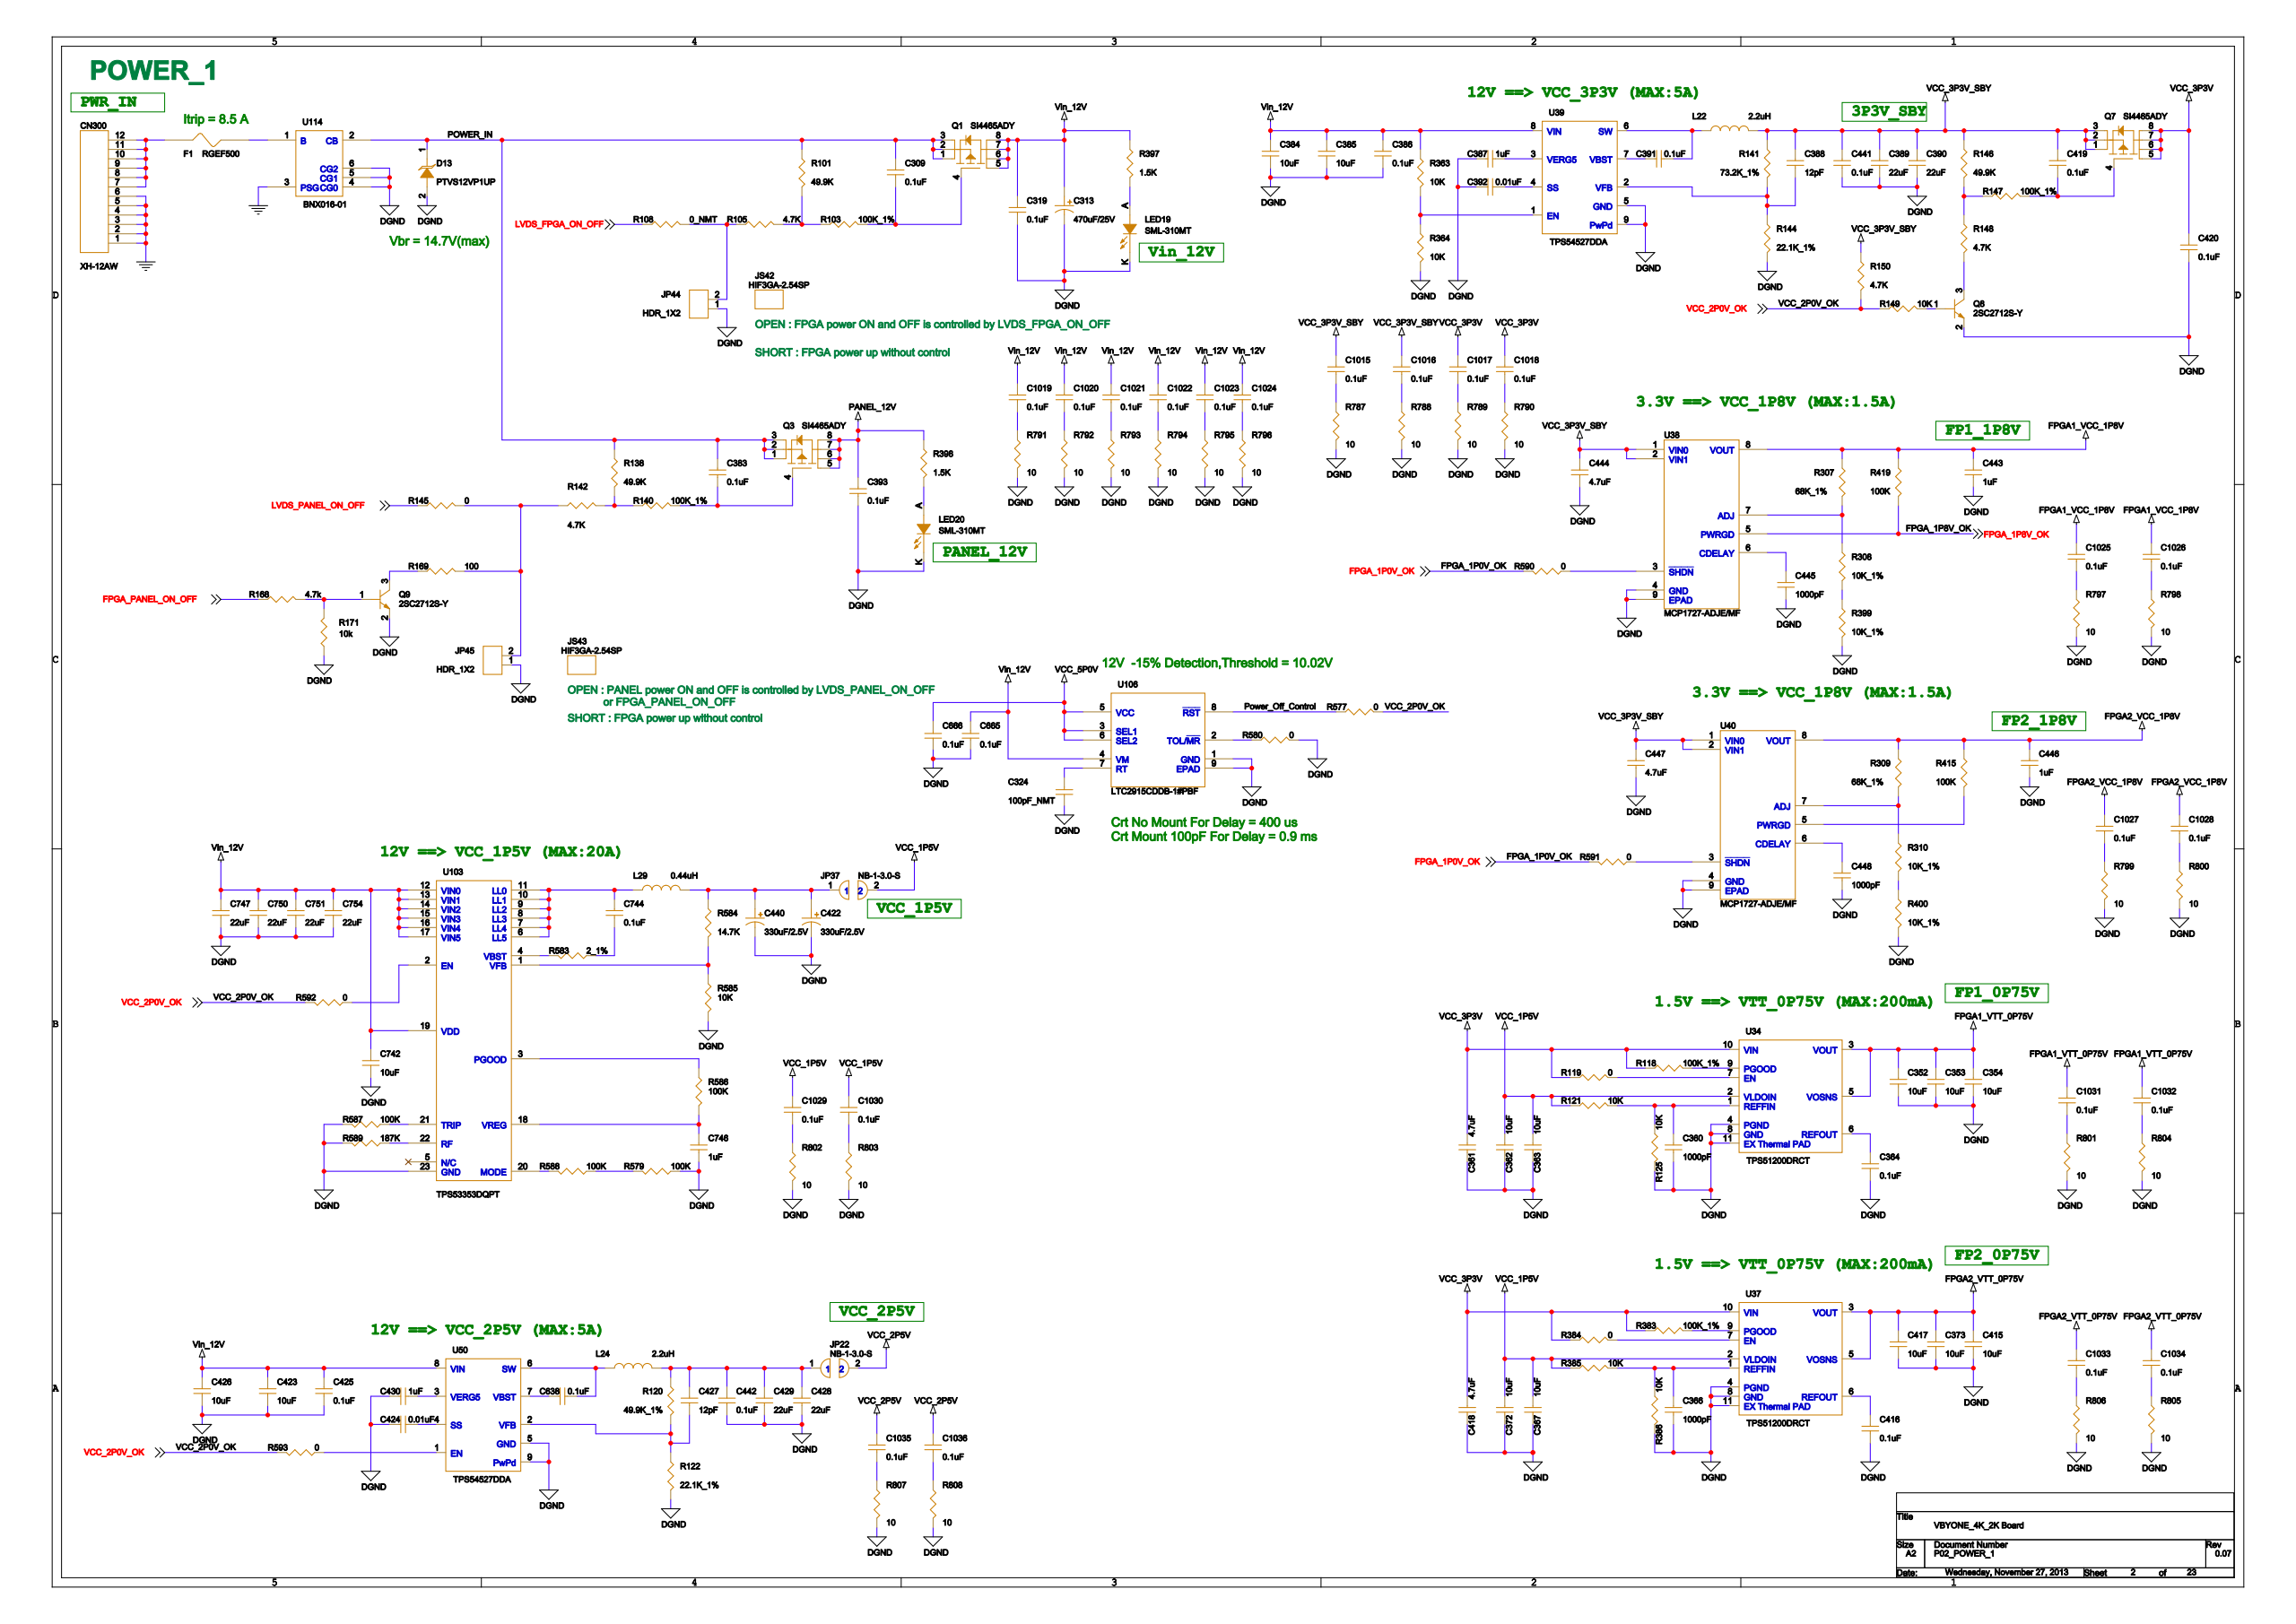Circuit board | Cadence Allegro | 1712 parts | 1495 nets | one sheet of the schematic
Parts on this sheet (reference | value | footprint):
C309 | 0.1uF | CRC1005RZAS
C313 | 470uF/25V | CEC100RZAS
C319 | 0.1uF | CRC1005RZAS
C324 | 100pF_NMT | CRC1608RZAS
C352 | 10uF | CRC2012RZAS
C353 | 10uF | CRC2012RZAS
C354 | 10uF | CRC2012RZAS
C360 | 1000pF | CRC1608RZAS
C361 | 4.7uF | CRC1608RZAS
C362 | 10uF | CRC2012RZAS
C363 | 10uF | CRC2012RZAS
C364 | 0.1uF | CRC1005RZAS
C366 | 1000pF | CRC1608RZAS
C367 | 10uF | CRC2012RZAS
C372 | 10uF | CRC2012RZAS
C373 | 10uF | CRC2012RZAS
C383 | 0.1uF | CRC1005RZAS
C384 | 10uF | CRC2012RZAS
C385 | 10uF | CRC2012RZAS
C386 | 0.1uF | CRC1005RZAS
C387 | 1uF | CRC1608RZAS
C388 | 12pF | CRC1608RZAS
C389 | 22uF | CRC3225RZAS
C390 | 22uF | CRC3225RZAS
C391 | 0.1uF | CRC1005RZAS
C392 | 0.01uF | CRC1005RZAS
C393 | 0.1uF | CRC1005RZAS
C415 | 10uF | CRC2012RZAS
C416 | 0.1uF | CRC1005RZAS
C417 | 10uF | CRC2012RZAS
C418 | 4.7uF | CRC1608RZAS
C419 | 0.1uF | CRC1005RZAS
C420 | 0.1uF | CRC1005RZAS
C422 | 330uF/2.5V | CEC3528RZAS
C423 | 10uF | CRC2012RZAS
C424 | 0.01uF | CRC1005RZAS
C425 | 0.1uF | CRC1005RZAS
C426 | 10uF | CRC2012RZAS
C427 | 12pF | CRC1608RZAS
C428 | 22uF | CRC3225RZAS
C429 | 22uF | CRC3225RZAS
C430 | 1uF | CRC1608RZAS
C440 | 330uF/2.5V | CEC3528RZAS
C441 | 0.1uF | CRC1005RZAS
C442 | 0.1uF | CRC1005RZAS
C443 | 1uF | CRC1608RZAS
C444 | 4.7uF | CRC1608RZAS
C445 | 1000pF | CRC1608RZAS
C446 | 1uF | CRC1608RZAS
C447 | 4.7uF | CRC1608RZAS
C448 | 1000pF | CRC1608RZAS
C638 | 0.1uF | CRC1005RZAS
C665 | 0.1uF | CRC1005RZAS
C666 | 0.1uF | CRC1005RZAS
C742 | 10uF | CRC2012RZAS
C744 | 0.1uF | CRC1005RZAS
C746 | 1uF | CRC1608RZAS
C747 | 22uF | CRC3225RZAS
C750 | 22uF | CRC3225RZAS
C751 | 22uF | CRC3225RZAS
C754 | 22uF | CRC3225RZAS
C1015 | 0.1uF | CRC1005RZAS
C1016 | 0.1uF | CRC1005RZAS
C1017 | 0.1uF | CRC1005RZAS
C1018 | 0.1uF | CRC1005RZAS
C1019 | 0.1uF | CRC1005RZAS
C1020 | 0.1uF | CRC1005RZAS
C1021 | 0.1uF | CRC1005RZAS
C1022 | 0.1uF | CRC1005RZAS
C1023 | 0.1uF | CRC1005RZAS
C1024 | 0.1uF | CRC1005RZAS
C1025 | 0.1uF | CRC1005RZAS
C1026 | 0.1uF | CRC1005RZAS
C1027 | 0.1uF | CRC1005RZAS
C1028 | 0.1uF | CRC1005RZAS
C1029 | 0.1uF | CRC1005RZAS
C1030 | 0.1uF | CRC1005RZAS
C1031 | 0.1uF | CRC1005RZAS
C1032 | 0.1uF | CRC1005RZAS
C1033 | 0.1uF | CRC1005RZAS
C1034 | 0.1uF | CRC1005RZAS
C1035 | 0.1uF | CRC1005RZAS
C1036 | 0.1uF | CRC1005RZAS
CN300 | XH-12AW | CAD012LKAS
D13 | PTVS12VP1UP | DIC002RZIS-2
F1 | RGEF500 | FLD002RZBS
JP22 | NB-1-3.0-S | CUTLAND35
JP37 | NB-1-3.0-S | CUTLAND35
JP44 | HDR_1X2 | CND002LLBS
JP45 | HDR_1X2 | CND002LLBS
L22 | 2.2uH | LSC5247RZAS
L24 | 2.2uH | LSC5247RZAS
L29 | 0.44uH | LSC002RZOS
LED19 | SML-310MT | LEC1608RZAS
LED20 | SML-310MT | LEC1608RZAS
Q1 | SI4465ADY | SOC008RHAS
Q3 | SI4465ADY | SOC008RHAS
Q7 | SI4465ADY | SOC008RHAS
Q8 | 2SC2712S-Y | TRC003RZCS
Q9 | 2SC2712S-Y | TRC003RZCS
R101 | 49.9K | CRC1608RZAS
R103 | 100K_1% | CRC1608RZAS
R105 | 4.7K | CRC1005RZAS
R108 | 0_NMT | CRC1608RZAS
R118 | 100K_1% | CRC1608RZAS
R119 | 0 | CRC1608RZAS
R120 | 49.9K_1% | CRC1608RZAS
R121 | 10K | CRC1005RZAS
R122 | 22.1K_1% | CRC1608RZAS
R125 | 10K | CRC1005RZAS
R138 | 49.9K | CRC1608RZAS
R140 | 100K_1% | CRC1608RZAS
R141 | 73.2K_1% | CRC1608RZAS
R142 | 4.7K | CRC1005RZAS
R144 | 22.1K_1% | CRC1608RZAS
R145 | 0 | CRC1608RZAS
R146 | 49.9K | CRC1608RZAS
R147 | 100K_1% | CRC1608RZAS
R148 | 4.7K | CRC1005RZAS
R149 | 10K | CRC1005RZAS
R150 | 4.7K | CRC1005RZAS
R168 | 4.7K | CRC1005RZAS
R169 | 100 | CRC1005RZAS
R171 | 10K | CRC1005RZAS
R307 | 68K_1% | CRC1608RZAS
R308 | 10K_1% | CRC1005RZAS
R309 | 68K_1% | CRC1608RZAS
R310 | 10K_1% | CRC1005RZAS
R363 | 10K | CRC1005RZAS
R364 | 10K | CRC1005RZAS
R383 | 100K_1% | CRC1608RZAS
R384 | 0 | CRC1608RZAS
R385 | 10K | CRC1005RZAS
R386 | 10K | CRC1005RZAS
R397 | 1.5K | CRC1608RZAS
R398 | 1.5K | CRC1608RZAS
R399 | 10K_1% | CRC1005RZAS
R400 | 10K_1% | CRC1005RZAS
R415 | 100K | CRC1608RZAS
R419 | 100K | CRC1608RZAS
R577 | 0 | CRC1608RZAS
R579 | 100K | CRC1608RZAS
R580 | 0 | CRC1608RZAS
R583 | 2_1% | CRC1608RZAS
R584 | 14.7K | CRC1608RZAS
R585 | 10K | CRC1005RZAS
R586 | 100K | CRC1608RZAS
R587 | 100K | CRC1608RZAS
R588 | 100K | CRC1608RZAS
R589 | 187K | CRC1608RZAS
R590 | 0 | CRC1608RZAS
R591 | 0 | CRC1608RZAS
R592 | 0 | CRC1608RZAS
R593 | 0 | CRC1608RZAS
R787 | 10 | CRC1005RZAS
R788 | 10 | CRC1005RZAS
R789 | 10 | CRC1005RZAS
R790 | 10 | CRC1005RZAS
R791 | 10 | CRC1005RZAS
R792 | 10 | CRC1005RZAS
R793 | 10 | CRC1005RZAS
R794 | 10 | CRC1005RZAS
R795 | 10 | CRC1005RZAS
R796 | 10 | CRC1005RZAS
R797 | 10 | CRC1005RZAS
R798 | 10 | CRC1005RZAS
R799 | 10 | CRC1005RZAS
R800 | 10 | CRC1005RZAS
R801 | 10 | CRC1005RZAS
R802 | 10 | CRC1005RZAS
R803 | 10 | CRC1005RZAS
R804 | 10 | CRC1005RZAS
R805 | 10 | CRC1005RZAS
R806 | 10 | CRC1005RZAS
R807 | 10 | CRC1005RZAS
R808 | 10 | CRC1005RZAS
U34 | TPS51200DRCT | QFN010RCAS
U37 | TPS51200DRCT | QFN010RCAS
U38 | MCP1727-ADJE/MF | SOC008REDS
U39 | TPS54527DDA | SOC008RHBS
U40 | MCP1727-ADJE/MF | SOC008REDS
U50 | TPS54527DDA | SOC008RHBS
U103 | TPS53353DQPT | SOC022RCAS
U106 | LTC2915CDDB-1#PBF | SOC008RCDS
U114 | BNX016-01 | FLD006LKAS
Nets of these parts (net: part-pin ...):
VCC_3P3V: C361-1 C418-1 C420-1 C1017-1 C1018-1 Q7-5 Q7-6 Q7-7 Q7-8 R118-1 R119-1 R383-1 R384-1 U34-10 U37-10
DGND: C313-2 C319-2 C324-1 C352-2 C353-2 C354-2 C360-2 C361-2 C362-2 C363-2 C364-2 C366-2 C367-2 C372-2 C373-2 C384-2 C385-2 C386-2 C387-1 C389-2 C390-2 C392-1 C393-2 C415-2 C416-2 C417-2 C418-2 C420-2 C422-2 C423-2 C424-1 C425-2 C426-2 C428-2 C429-2 C430-1 C440-2 C441-2 C442-2 C443-2 C444-2 C445-2 C446-2 C447-2 C448-2 C665-1 C666-1 C742-2 C746-2 C747-2 C750-2 C751-2 C754-2 D13-2 JP44-1 JP45-1 LED19-K LED20-K Q8-2 Q9-2 R122-2 R125-2 R144-2 R171-1 R364-2 R386-2 R399-2 R400-2 R579-1 R580-2 R585-2 R587-2 R589-2 R787-2 R788-2 R789-2 R790-2 R791-2 R792-2 R793-2 R794-2 R795-2 R796-2 R797-2 R798-2 R799-2 R800-2 R801-2 R802-2 R803-2 R804-2 R805-2 R806-2 R807-2 R808-2 U34-4 U34-8 U34-11 U37-4 U37-8 U37-11 U38-4 U38-9 U39-5 U39-9 U40-4 U40-9 U50-5 U50-9 U106-1 U106-9 U114-4 U114-5 U114-6 U103-23
VCC_1P5V: C362-1 C363-1 C367-1 C372-1 C1029-1 C1030-1 JP37-2 R121-1 R385-1 U34-2 U37-2
VCC_3P3V_SBY: C388-1 C389-1 C390-1 C419-1 C441-1 C444-1 C447-1 C1015-1 C1016-1 L22-2 Q7-1 Q7-2 Q7-3 R141-1 R146-1 R150-1 U38-1 U38-2 U40-1 U40-2
N19944978: C1015-2 R787-1
N19945009: C1016-2 R788-1
N19945053: C1017-2 R789-1
N19945065: C1018-2 R790-1
VIN_12V: C313-1 C319-1 C384-1 C385-1 C386-1 C423-1 C425-1 C426-1 C665-2 C742-1 C747-1 C750-1 C751-1 C754-1 C1019-1 C1020-1 C1021-1 C1022-1 C1023-1 C1024-1 Q1-5 Q1-6 Q1-7 Q1-8 R363-1 R397-1 U39-8 U50-8 U106-4 U103-12 U103-13 U103-14 U103-15 U103-16 U103-17 U103-19
N19940256: C1019-2 R791-1
N19941245: C1020-2 R792-1
N19941511: C1021-2 R793-1
N19941779: C1022-2 R794-1
N19941808: C1023-2 R795-1
N19941837: C1024-2 R796-1
FPGA1_VCC_1P8V: C443-1 C1025-1 C1026-1 R307-1 R419-1 U38-8
N19947558: C1025-2 R797-1
N19947572: C1026-2 R798-1
FPGA2_VCC_1P8V: C446-1 C1027-1 C1028-1 R309-1 R415-1 U40-8
N19948575: C1027-2 R799-1
N19948579: C1028-2 R800-1
N19951656: C1029-2 R802-1
N19951688: C1030-2 R803-1
FPGA1_VTT_0P75V: C352-1 C353-1 C354-1 C1031-1 C1032-1 U34-3 U34-5
N19948889: C1031-2 R801-1
N19948895: C1032-2 R804-1
FPGA2_VTT_0P75V: C373-1 C415-1 C417-1 C1033-1 C1034-1 U37-3 U37-5
N19949219: C1033-2 R806-1
N19949213: C1034-2 R805-1
VCC_2P5V: C1035-1 C1036-1 JP22-2
N19951132: C1035-2 R807-1
N19951164: C1036-2 R808-1
POWER_IN: C309-1 C383-1 D13-1 Q1-1 Q1-2 Q1-3 Q3-1 Q3-2 Q3-3 R101-1 R138-1 U114-2
N15783925: C309-2 Q1-4 R103-2
N16970548: C364-1 U34-6
N17163997: C383-2 Q3-4 R140-2
N17322746: C391-1 U39-7
N17322740: C391-2 L22-1 U39-6
PANEL_12V: C393-1 Q3-5 Q3-6 Q3-7 Q3-8 R398-1
N18162801: C416-1 U37-6
N17546760: C419-2 Q7-4 R147-2
N18317834: C427-1 C428-1 C429-1 C442-1 JP22-1 L24-2 R120-1
N18317826: C638-1 U50-7
N18317824: C638-2 L24-1 U50-6
VCC_5P0V: C666-2 U106-3 U106-5 U106-6
N17322991: C387-2 U39-3
N18317806: C430-2 U50-3
N16970580: C360-1 R121-2 R125-1 U34-1
N18162813: C366-1 R385-2 R386-1 U37-1
N18318720: C445-1 U38-6
N18320450: C448-1 U40-6
N18312599: C744-1 L29-1 U103-6 U103-7 U103-8 U103-9 U103-10 U103-11
N18312643: C744-2 R583-1
N18161409: C324-2 U106-7
N18312681: C746-1 R586-2 U103-18
N17322734: C388-2 R141-2 R144-1 U39-2
N18317842: C427-2 R120-2 R122-1 U50-2
N17322989: C392-2 U39-4
N18317822: C424-2 U50-4
N18312559: C422-1 C440-1 JP37-1 L29-2 R584-1
LVDS_PANEL_ON_OFF: R145-1
LVDS_FPGA_ON_OFF: R108-1
GND: CN300-1 CN300-2 CN300-3 CN300-4 CN300-5 CN300-6 U114-3
N15783757: CN300-7 CN300-8 CN300-9 CN300-10 CN300-11 CN300-12 F1-1
N18434432: F1-2 U114-1
N18311244: JP44-2 R105-1 R108-2
N18311238: JP45-2 R142-1 R145-2 R169-2
N18306479: LED19-A R397-2
N18307386: LED20-A R398-2
N17546833: Q8-1 R149-2
N17546812: Q8-3 R148-2
N19339127: Q9-1 R168-2 R171-2
N19339892: Q9-3 R169-1
N16970708: R119-2 U34-7
FPGA_1P8V_OK: R419-2 U38-5
N18162935: R384-2 U37-7
POWER_OFF_CONTROL: R577-1 U106-8
VCC_2P0V_OK: R149-1 R150-2 R577-2 R592-2 R593-2
N18161338: R580-1 U106-2
N18318745: R590-1 U38-3
FPGA_1P0V_OK: R590-2 R591-2
N18320471: R591-1 U40-3
N18312513: R592-1 U103-2
N18318066: R593-1 U50-1
N15783909: R101-2 R103-1 R105-2
N17164003: R138-2 R140-1 R142-2
N17546756: R146-2 R147-1 R148-1
N16970819: R118-2 U34-9
N18163050: R383-2 U37-9
FPGA_PANEL_ON_OFF: R168-1
N17549104: R363-2 R364-1 U39-1
N18312673: R584-2 R585-1 U103-1
N18318724: R307-2 R308-1 U38-7
N18318756: R308-2 R399-1
N18320454: R309-2 R310-1 U40-7
N18320478: R310-2 R400-1
N18415573: R415-2 U40-5
N18312451: R579-2 R588-1
N18312709: R586-1 U103-3
N18312758: R587-1 U103-21
N18312685: R588-2 U103-20
N18312641: R583-2 U103-4
N18312748: R589-1 U103-22